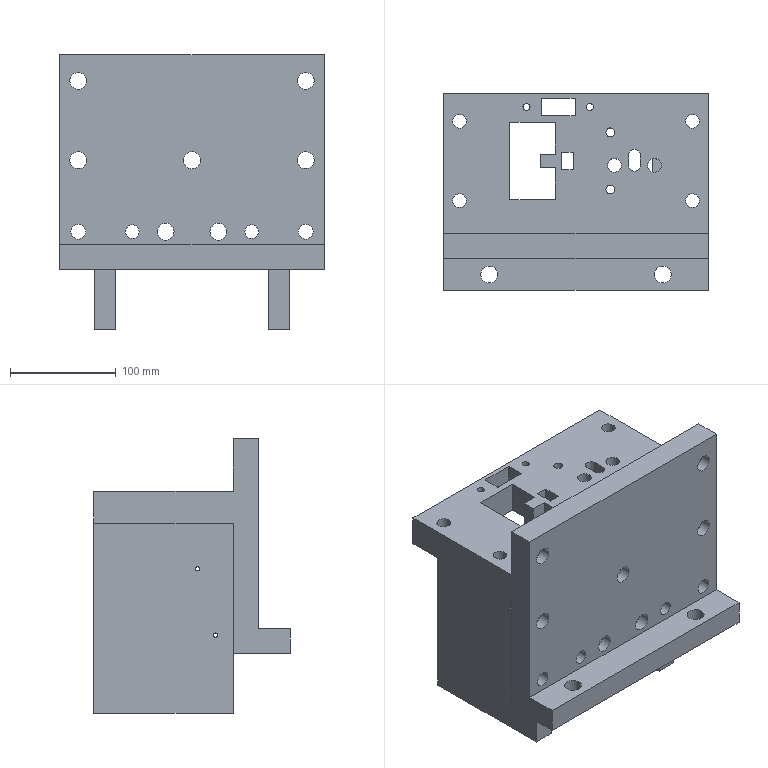Part | STEP file | GA KHUON COI CO LOGO.dwg | 1 solid | 147 faces | box 250 x 186 x 260 mm | volume 3082669 mm3 | cylinder 86 | plane 53 | cone 8 | commonest cylinder face diameters 16 x18 13 x16 23 x14 4.134 x8 10.106 x8 2 x4